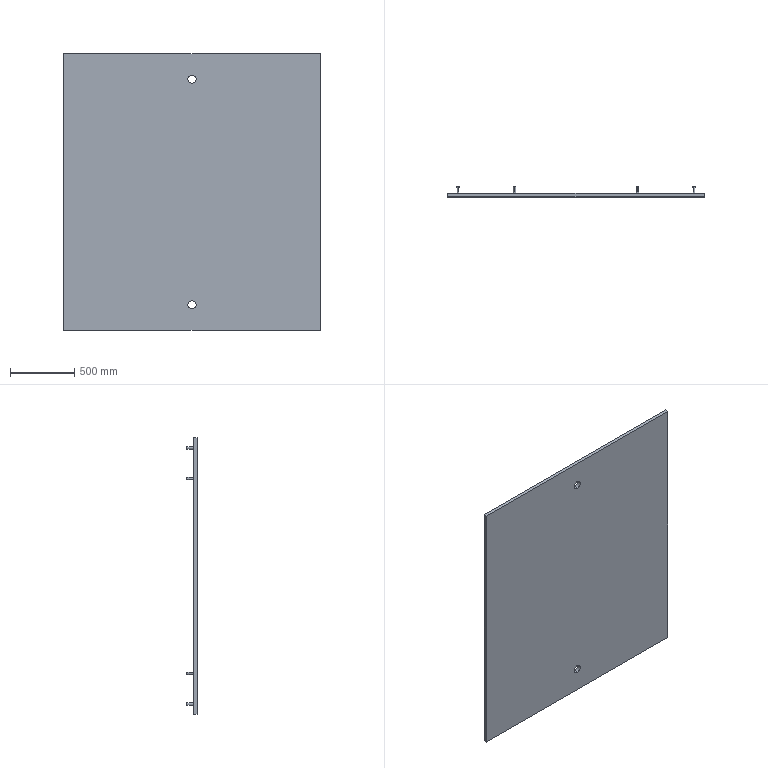Part | SolidWorks | features ICE 2, Extrusion 1 | 1 solid | 58 faces | box 2000 x 80 x 2160 mm | volume 129658308 mm3 | cylinder 36 | plane 22 | commonest cylinder face diameters 20 x32 64 x4
STEP:
#1=CARTESIAN_POINT('',(0.,0.,-848.));
#2=VERTEX_POINT('',#1);
#3=CARTESIAN_POINT('',(0.,0.,-912.));
#4=VERTEX_POINT('',#3);
#5=CARTESIAN_POINT('',(0.,0.,-880.));
#6=DIRECTION('',(0.,-1.,0.));
#7=DIRECTION('',(0.,0.,-1.));
#8=AXIS2_PLACEMENT_3D('',#5,#6,#7);
#9=CIRCLE('',#8,32.);
#10=EDGE_CURVE('',#2,#4,#9,.T.);
#11=ORIENTED_EDGE('',*,*,#10,.T.);
#12=CARTESIAN_POINT('',(0.,30.,-912.));
#13=VERTEX_POINT('',#12);
#14=CARTESIAN_POINT('',(0.,-10.,-912.));
#15=DIRECTION('',(0.,1.,0.));
#16=VECTOR('',#15,1000.);
#17=LINE('',#14,#16);
#18=EDGE_CURVE('',#4,#13,#17,.T.);
#19=ORIENTED_EDGE('',*,*,#18,.T.);
#20=CARTESIAN_POINT('',(0.,30.,-848.));
#21=VERTEX_POINT('',#20);
#22=CARTESIAN_POINT('',(0.,30.,-880.));
#23=DIRECTION('',(0.,1.,0.));
#24=DIRECTION('',(0.,0.,1.));
#25=AXIS2_PLACEMENT_3D('',#22,#23,#24);
#26=CIRCLE('',#25,32.);
#27=EDGE_CURVE('',#13,#21,#26,.T.);
#28=ORIENTED_EDGE('',*,*,#27,.T.);
#29=CARTESIAN_POINT('',(0.,-10.,-848.));
#30=DIRECTION('',(0.,1.,0.));
#31=VECTOR('',#30,1000.);
#32=LINE('',#29,#31);
#33=EDGE_CURVE('',#2,#21,#32,.T.);
#34=ORIENTED_EDGE('',*,*,#33,.F.);
#35=EDGE_LOOP('',(#11,#19,#28,#34));
#36=FACE_OUTER_BOUND('',#35,.T.);
#37=CARTESIAN_POINT('',(0.,-10.,-880.));
#38=DIRECTION('',(0.,1.,0.));
#39=DIRECTION('',(0.,0.,1.));
#40=AXIS2_PLACEMENT_3D('',#37,#38,#39);
#41=CYLINDRICAL_SURFACE('',#40,32.);
#42=ADVANCED_FACE('',(#36),#41,.F.);
#43=CARTESIAN_POINT('',(0.,0.,912.));
#44=VERTEX_POINT('',#43);
#45=CARTESIAN_POINT('',(0.,0.,848.));
#46=VERTEX_POINT('',#45);
#47=CARTESIAN_POINT('',(0.,0.,880.));
#48=DIRECTION('',(0.,-1.,0.));
#49=DIRECTION('',(0.,0.,-1.));
#50=AXIS2_PLACEMENT_3D('',#47,#48,#49);
#51=CIRCLE('',#50,32.);
#52=EDGE_CURVE('',#44,#46,#51,.T.);
#53=ORIENTED_EDGE('',*,*,#52,.T.);
#54=CARTESIAN_POINT('',(0.,30.,848.));
#55=VERTEX_POINT('',#54);
#56=CARTESIAN_POINT('',(0.,-10.,848.));
#57=DIRECTION('',(0.,1.,0.));
#58=VECTOR('',#57,1000.);
#59=LINE('',#56,#58);
#60=EDGE_CURVE('',#46,#55,#59,.T.);
#61=ORIENTED_EDGE('',*,*,#60,.T.);
#62=CARTESIAN_POINT('',(0.,30.,912.));
#63=VERTEX_POINT('',#62);
#64=CARTESIAN_POINT('',(0.,30.,880.));
#65=DIRECTION('',(0.,1.,0.));
#66=DIRECTION('',(0.,0.,1.));
#67=AXIS2_PLACEMENT_3D('',#64,#65,#66);
#68=CIRCLE('',#67,32.);
#69=EDGE_CURVE('',#55,#63,#68,.T.);
#70=ORIENTED_EDGE('',*,*,#69,.T.);
#71=CARTESIAN_POINT('',(0.,-10.,912.));
#72=DIRECTION('',(0.,1.,0.));
#73=VECTOR('',#72,1000.);
#74=LINE('',#71,#73);
#75=EDGE_CURVE('',#44,#63,#74,.T.);
#76=ORIENTED_EDGE('',*,*,#75,.F.);
#77=EDGE_LOOP('',(#53,#61,#70,#76));
#78=FACE_OUTER_BOUND('',#77,.T.);
#79=CARTESIAN_POINT('',(0.,-10.,880.));
#80=DIRECTION('',(0.,1.,0.));
#81=DIRECTION('',(0.,0.,1.));
#82=AXIS2_PLACEMENT_3D('',#79,#80,#81);
#83=CYLINDRICAL_SURFACE('',#82,32.);
#84=ADVANCED_FACE('',(#78),#83,.F.);
#85=CARTESIAN_POINT('',(-920.,80.,1010.));
#86=VERTEX_POINT('',#85);
#87=CARTESIAN_POINT('',(-920.,80.,990.));
#88=VERTEX_POINT('',#87);
#89=CARTESIAN_POINT('',(-920.,80.,1000.));
#90=DIRECTION('',(0.,1.,0.));
#91=DIRECTION('',(0.,0.,-1.));
#92=AXIS2_PLACEMENT_3D('',#89,#90,#91);
#93=CIRCLE('',#92,10.);
#94=EDGE_CURVE('',#86,#88,#93,.T.);
#95=ORIENTED_EDGE('',*,*,#94,.F.);
#96=CARTESIAN_POINT('',(-920.,30.,1010.));
#97=VERTEX_POINT('',#96);
#98=CARTESIAN_POINT('',(-920.,80.,1010.));
#99=DIRECTION('',(0.,-1.,0.));
#100=VECTOR('',#99,1000.);
#101=LINE('',#98,#100);
#102=EDGE_CURVE('',#86,#97,#101,.T.);
#103=ORIENTED_EDGE('',*,*,#102,.T.);
#104=CARTESIAN_POINT('',(-920.,30.,990.));
#105=VERTEX_POINT('',#104);
#106=CARTESIAN_POINT('',(-920.,30.,1000.));
#107=DIRECTION('',(0.,1.,0.));
#108=DIRECTION('',(0.,0.,-1.));
#109=AXIS2_PLACEMENT_3D('',#106,#107,#108);
#110=CIRCLE('',#109,10.);
#111=EDGE_CURVE('',#97,#105,#110,.T.);
#112=ORIENTED_EDGE('',*,*,#111,.T.);
#113=CARTESIAN_POINT('',(-920.,80.,990.));
#114=DIRECTION('',(0.,-1.,0.));
#115=VECTOR('',#114,1000.);
#116=LINE('',#113,#115);
#117=EDGE_CURVE('',#88,#105,#116,.T.);
#118=ORIENTED_EDGE('',*,*,#117,.F.);
#119=EDGE_LOOP('',(#95,#103,#112,#118));
#120=FACE_OUTER_BOUND('',#119,.T.);
#121=CARTESIAN_POINT('',(-920.,80.,1000.));
#122=DIRECTION('',(0.,-1.,0.));
#123=DIRECTION('',(0.,0.,-1.));
#124=AXIS2_PLACEMENT_3D('',#121,#122,#123);
#125=CYLINDRICAL_SURFACE('',#124,10.);
#126=ADVANCED_FACE('',(#120),#125,.T.);
#127=CARTESIAN_POINT('',(-920.,80.,770.));
#128=VERTEX_POINT('',#127);
#129=CARTESIAN_POINT('',(-920.,80.,750.));
#130=VERTEX_POINT('',#129);
#131=CARTESIAN_POINT('',(-920.,80.,760.));
#132=DIRECTION('',(0.,1.,0.));
#133=DIRECTION('',(0.,0.,-1.));
#134=AXIS2_PLACEMENT_3D('',#131,#132,#133);
#135=CIRCLE('',#134,10.);
#136=EDGE_CURVE('',#128,#130,#135,.T.);
#137=ORIENTED_EDGE('',*,*,#136,.F.);
#138=CARTESIAN_POINT('',(-920.,30.,770.));
#139=VERTEX_POINT('',#138);
#140=CARTESIAN_POINT('',(-920.,80.,770.));
#141=DIRECTION('',(0.,-1.,0.));
#142=VECTOR('',#141,1000.);
#143=LINE('',#140,#142);
#144=EDGE_CURVE('',#128,#139,#143,.T.);
#145=ORIENTED_EDGE('',*,*,#144,.T.);
#146=CARTESIAN_POINT('',(-920.,30.,750.));
#147=VERTEX_POINT('',#146);
#148=CARTESIAN_POINT('',(-920.,30.,760.));
#149=DIRECTION('',(0.,1.,0.));
#150=DIRECTION('',(0.,0.,-1.));
#151=AXIS2_PLACEMENT_3D('',#148,#149,#150);
#152=CIRCLE('',#151,10.);
#153=EDGE_CURVE('',#139,#147,#152,.T.);
#154=ORIENTED_EDGE('',*,*,#153,.T.);
#155=CARTESIAN_POINT('',(-920.,80.,750.));
#156=DIRECTION('',(0.,-1.,0.));
#157=VECTOR('',#156,1000.);
#158=LINE('',#155,#157);
#159=EDGE_CURVE('',#130,#147,#158,.T.);
#160=ORIENTED_EDGE('',*,*,#159,.F.);
#161=EDGE_LOOP('',(#137,#145,#154,#160));
#162=FACE_OUTER_BOUND('',#161,.T.);
#163=CARTESIAN_POINT('',(-920.,80.,760.));
#164=DIRECTION('',(0.,-1.,0.));
#165=DIRECTION('',(0.,0.,-1.));
#166=AXIS2_PLACEMENT_3D('',#163,#164,#165);
#167=CYLINDRICAL_SURFACE('',#166,10.);
#168=ADVANCED_FACE('',(#162),#167,.T.);
#169=CARTESIAN_POINT('',(-480.,80.,1010.));
#170=VERTEX_POINT('',#169);
#171=CARTESIAN_POINT('',(-480.,80.,990.));
#172=VERTEX_POINT('',#171);
#173=CARTESIAN_POINT('',(-480.,80.,1000.));
#174=DIRECTION('',(0.,1.,0.));
#175=DIRECTION('',(0.,0.,-1.));
#176=AXIS2_PLACEMENT_3D('',#173,#174,#175);
#177=CIRCLE('',#176,10.);
#178=EDGE_CURVE('',#170,#172,#177,.T.);
#179=ORIENTED_EDGE('',*,*,#178,.F.);
#180=CARTESIAN_POINT('',(-480.,30.,1010.));
#181=VERTEX_POINT('',#180);
#182=CARTESIAN_POINT('',(-480.,80.,1010.));
#183=DIRECTION('',(0.,-1.,0.));
#184=VECTOR('',#183,1000.);
#185=LINE('',#182,#184);
#186=EDGE_CURVE('',#170,#181,#185,.T.);
#187=ORIENTED_EDGE('',*,*,#186,.T.);
#188=CARTESIAN_POINT('',(-480.,30.,990.));
#189=VERTEX_POINT('',#188);
#190=CARTESIAN_POINT('',(-480.,30.,1000.));
#191=DIRECTION('',(0.,1.,0.));
#192=DIRECTION('',(0.,0.,-1.));
#193=AXIS2_PLACEMENT_3D('',#190,#191,#192);
#194=CIRCLE('',#193,10.);
#195=EDGE_CURVE('',#181,#189,#194,.T.);
#196=ORIENTED_EDGE('',*,*,#195,.T.);
#197=CARTESIAN_POINT('',(-480.,80.,990.));
#198=DIRECTION('',(0.,-1.,0.));
#199=VECTOR('',#198,1000.);
#200=LINE('',#197,#199);
#201=EDGE_CURVE('',#172,#189,#200,.T.);
#202=ORIENTED_EDGE('',*,*,#201,.F.);
#203=EDGE_LOOP('',(#179,#187,#196,#202));
#204=FACE_OUTER_BOUND('',#203,.T.);
#205=CARTESIAN_POINT('',(-480.,80.,1000.));
#206=DIRECTION('',(0.,-1.,0.));
#207=DIRECTION('',(0.,0.,-1.));
#208=AXIS2_PLACEMENT_3D('',#205,#206,#207);
#209=CYLINDRICAL_SURFACE('',#208,10.);
#210=ADVANCED_FACE('',(#204),#209,.T.);
#211=CARTESIAN_POINT('',(-480.,80.,770.));
#212=VERTEX_POINT('',#211);
#213=CARTESIAN_POINT('',(-480.,80.,750.));
#214=VERTEX_POINT('',#213);
#215=CARTESIAN_POINT('',(-480.,80.,760.));
#216=DIRECTION('',(0.,1.,0.));
#217=DIRECTION('',(0.,0.,-1.));
#218=AXIS2_PLACEMENT_3D('',#215,#216,#217);
#219=CIRCLE('',#218,10.);
#220=EDGE_CURVE('',#212,#214,#219,.T.);
#221=ORIENTED_EDGE('',*,*,#220,.F.);
#222=CARTESIAN_POINT('',(-480.,30.,770.));
#223=VERTEX_POINT('',#222);
#224=CARTESIAN_POINT('',(-480.,80.,770.));
#225=DIRECTION('',(0.,-1.,0.));
#226=VECTOR('',#225,1000.);
#227=LINE('',#224,#226);
#228=EDGE_CURVE('',#212,#223,#227,.T.);
#229=ORIENTED_EDGE('',*,*,#228,.T.);
#230=CARTESIAN_POINT('',(-480.,30.,750.));
#231=VERTEX_POINT('',#230);
#232=CARTESIAN_POINT('',(-480.,30.,760.));
#233=DIRECTION('',(0.,1.,0.));
#234=DIRECTION('',(0.,0.,-1.));
#235=AXIS2_PLACEMENT_3D('',#232,#233,#234);
#236=CIRCLE('',#235,10.);
#237=EDGE_CURVE('',#223,#231,#236,.T.);
#238=ORIENTED_EDGE('',*,*,#237,.T.);
#239=CARTESIAN_POINT('',(-480.,80.,750.));
#240=DIRECTION('',(0.,-1.,0.));
#241=VECTOR('',#240,1000.);
#242=LINE('',#239,#241);
#243=EDGE_CURVE('',#214,#231,#242,.T.);
#244=ORIENTED_EDGE('',*,*,#243,.F.);
#245=EDGE_LOOP('',(#221,#229,#238,#244));
#246=FACE_OUTER_BOUND('',#245,.T.);
#247=CARTESIAN_POINT('',(-480.,80.,760.));
#248=DIRECTION('',(0.,-1.,0.));
#249=DIRECTION('',(0.,0.,-1.));
#250=AXIS2_PLACEMENT_3D('',#247,#248,#249);
#251=CYLINDRICAL_SURFACE('',#250,10.);
#252=ADVANCED_FACE('',(#246),#251,.T.);
#253=CARTESIAN_POINT('',(480.,80.,770.));
#254=VERTEX_POINT('',#253);
#255=CARTESIAN_POINT('',(480.,80.,750.));
#256=VERTEX_POINT('',#255);
#257=CARTESIAN_POINT('',(480.,80.,760.));
#258=DIRECTION('',(0.,1.,0.));
#259=DIRECTION('',(0.,0.,1.));
#260=AXIS2_PLACEMENT_3D('',#257,#258,#259);
#261=CIRCLE('',#260,10.);
#262=EDGE_CURVE('',#254,#256,#261,.T.);
#263=ORIENTED_EDGE('',*,*,#262,.F.);
#264=CARTESIAN_POINT('',(480.,30.,770.));
#265=VERTEX_POINT('',#264);
#266=CARTESIAN_POINT('',(480.,80.,770.));
#267=DIRECTION('',(0.,-1.,0.));
#268=VECTOR('',#267,1000.);
#269=LINE('',#266,#268);
#270=EDGE_CURVE('',#254,#265,#269,.T.);
#271=ORIENTED_EDGE('',*,*,#270,.T.);
#272=CARTESIAN_POINT('',(480.,30.,750.));
#273=VERTEX_POINT('',#272);
#274=CARTESIAN_POINT('',(480.,30.,760.));
#275=DIRECTION('',(0.,1.,0.));
#276=DIRECTION('',(0.,0.,-1.));
#277=AXIS2_PLACEMENT_3D('',#274,#275,#276);
#278=CIRCLE('',#277,10.);
#279=EDGE_CURVE('',#265,#273,#278,.T.);
#280=ORIENTED_EDGE('',*,*,#279,.T.);
#281=CARTESIAN_POINT('',(480.,80.,750.));
#282=DIRECTION('',(0.,-1.,0.));
#283=VECTOR('',#282,1000.);
#284=LINE('',#281,#283);
#285=EDGE_CURVE('',#256,#273,#284,.T.);
#286=ORIENTED_EDGE('',*,*,#285,.F.);
#287=EDGE_LOOP('',(#263,#271,#280,#286));
#288=FACE_OUTER_BOUND('',#287,.T.);
#289=CARTESIAN_POINT('',(480.,80.,760.));
#290=DIRECTION('',(0.,-1.,0.));
#291=DIRECTION('',(0.,0.,-1.));
#292=AXIS2_PLACEMENT_3D('',#289,#290,#291);
#293=CYLINDRICAL_SURFACE('',#292,10.);
#294=ADVANCED_FACE('',(#288),#293,.T.);
#295=CARTESIAN_POINT('',(480.,80.,1010.));
#296=VERTEX_POINT('',#295);
#297=CARTESIAN_POINT('',(480.,80.,990.));
#298=VERTEX_POINT('',#297);
#299=CARTESIAN_POINT('',(480.,80.,1000.));
#300=DIRECTION('',(0.,1.,0.));
#301=DIRECTION('',(0.,0.,1.));
#302=AXIS2_PLACEMENT_3D('',#299,#300,#301);
#303=CIRCLE('',#302,10.);
#304=EDGE_CURVE('',#296,#298,#303,.T.);
#305=ORIENTED_EDGE('',*,*,#304,.F.);
#306=CARTESIAN_POINT('',(480.,30.,1010.));
#307=VERTEX_POINT('',#306);
#308=CARTESIAN_POINT('',(480.,80.,1010.));
#309=DIRECTION('',(0.,-1.,0.));
#310=VECTOR('',#309,1000.);
#311=LINE('',#308,#310);
#312=EDGE_CURVE('',#296,#307,#311,.T.);
#313=ORIENTED_EDGE('',*,*,#312,.T.);
#314=CARTESIAN_POINT('',(480.,30.,990.));
#315=VERTEX_POINT('',#314);
#316=CARTESIAN_POINT('',(480.,30.,1000.));
#317=DIRECTION('',(0.,1.,0.));
#318=DIRECTION('',(0.,0.,-1.));
#319=AXIS2_PLACEMENT_3D('',#316,#317,#318);
#320=CIRCLE('',#319,10.);
#321=EDGE_CURVE('',#307,#315,#320,.T.);
#322=ORIENTED_EDGE('',*,*,#321,.T.);
#323=CARTESIAN_POINT('',(480.,80.,990.));
#324=DIRECTION('',(0.,-1.,0.));
#325=VECTOR('',#324,1000.);
#326=LINE('',#323,#325);
#327=EDGE_CURVE('',#298,#315,#326,.T.);
#328=ORIENTED_EDGE('',*,*,#327,.F.);
#329=EDGE_LOOP('',(#305,#313,#322,#328));
#330=FACE_OUTER_BOUND('',#329,.T.);
#331=CARTESIAN_POINT('',(480.,80.,1000.));
#332=DIRECTION('',(0.,-1.,0.));
#333=DIRECTION('',(0.,0.,-1.));
#334=AXIS2_PLACEMENT_3D('',#331,#332,#333);
#335=CYLINDRICAL_SURFACE('',#334,10.);
#336=ADVANCED_FACE('',(#330),#335,.T.);
#337=CARTESIAN_POINT('',(920.,80.,770.));
#338=VERTEX_POINT('',#337);
#339=CARTESIAN_POINT('',(920.,80.,750.));
#340=VERTEX_POINT('',#339);
#341=CARTESIAN_POINT('',(920.,80.,760.));
#342=DIRECTION('',(0.,1.,0.));
#343=DIRECTION('',(0.,0.,1.));
#344=AXIS2_PLACEMENT_3D('',#341,#342,#343);
#345=CIRCLE('',#344,10.);
#346=EDGE_CURVE('',#338,#340,#345,.T.);
#347=ORIENTED_EDGE('',*,*,#346,.F.);
#348=CARTESIAN_POINT('',(920.,30.,770.));
#349=VERTEX_POINT('',#348);
#350=CARTESIAN_POINT('',(920.,80.,770.));
#351=DIRECTION('',(0.,-1.,0.));
#352=VECTOR('',#351,1000.);
#353=LINE('',#350,#352);
#354=EDGE_CURVE('',#338,#349,#353,.T.);
#355=ORIENTED_EDGE('',*,*,#354,.T.);
#356=CARTESIAN_POINT('',(920.,30.,750.));
#357=VERTEX_POINT('',#356);
#358=CARTESIAN_POINT('',(920.,30.,760.));
#359=DIRECTION('',(0.,1.,0.));
#360=DIRECTION('',(0.,0.,-1.));
#361=AXIS2_PLACEMENT_3D('',#358,#359,#360);
#362=CIRCLE('',#361,10.);
#363=EDGE_CURVE('',#349,#357,#362,.T.);
#364=ORIENTED_EDGE('',*,*,#363,.T.);
#365=CARTESIAN_POINT('',(920.,80.,750.));
#366=DIRECTION('',(0.,-1.,0.));
#367=VECTOR('',#366,1000.);
#368=LINE('',#365,#367);
#369=EDGE_CURVE('',#340,#357,#368,.T.);
#370=ORIENTED_EDGE('',*,*,#369,.F.);
#371=EDGE_LOOP('',(#347,#355,#364,#370));
#372=FACE_OUTER_BOUND('',#371,.T.);
#373=CARTESIAN_POINT('',(920.,80.,760.));
#374=DIRECTION('',(0.,-1.,0.));
#375=DIRECTION('',(0.,0.,-1.));
#376=AXIS2_PLACEMENT_3D('',#373,#374,#375);
#377=CYLINDRICAL_SURFACE('',#376,10.);
#378=ADVANCED_FACE('',(#372),#377,.T.);
#379=CARTESIAN_POINT('',(920.,80.,1010.));
#380=VERTEX_POINT('',#379);
#381=CARTESIAN_POINT('',(920.,80.,990.));
#382=VERTEX_POINT('',#381);
#383=CARTESIAN_POINT('',(920.,80.,1000.));
#384=DIRECTION('',(0.,1.,0.));
#385=DIRECTION('',(0.,0.,1.));
#386=AXIS2_PLACEMENT_3D('',#383,#384,#385);
#387=CIRCLE('',#386,10.);
#388=EDGE_CURVE('',#380,#382,#387,.T.);
#389=ORIENTED_EDGE('',*,*,#388,.F.);
#390=CARTESIAN_POINT('',(920.,30.,1010.));
#391=VERTEX_POINT('',#390);
#392=CARTESIAN_POINT('',(920.,80.,1010.));
#393=DIRECTION('',(0.,-1.,0.));
#394=VECTOR('',#393,1000.);
#395=LINE('',#392,#394);
#396=EDGE_CURVE('',#380,#391,#395,.T.);
#397=ORIENTED_EDGE('',*,*,#396,.T.);
#398=CARTESIAN_POINT('',(920.,30.,990.));
#399=VERTEX_POINT('',#398);
#400=CARTESIAN_POINT('',(920.,30.,1000.));
#401=DIRECTION('',(0.,1.,0.));
#402=DIRECTION('',(0.,0.,-1.));
#403=AXIS2_PLACEMENT_3D('',#400,#401,#402);
#404=CIRCLE('',#403,10.);
#405=EDGE_CURVE('',#391,#399,#404,.T.);
#406=ORIENTED_EDGE('',*,*,#405,.T.);
#407=CARTESIAN_POINT('',(920.,80.,990.));
#408=DIRECTION('',(0.,-1.,0.));
#409=VECTOR('',#408,1000.);
#410=LINE('',#407,#409);
#411=EDGE_CURVE('',#382,#399,#410,.T.);
#412=ORIENTED_EDGE('',*,*,#411,.F.);
#413=EDGE_LOOP('',(#389,#397,#406,#412));
#414=FACE_OUTER_BOUND('',#413,.T.);
#415=CARTESIAN_POINT('',(920.,80.,1000.));
#416=DIRECTION('',(0.,-1.,0.));
#417=DIRECTION('',(0.,0.,-1.));
#418=AXIS2_PLACEMENT_3D('',#415,#416,#417);
#419=CYLINDRICAL_SURFACE('',#418,10.);
#420=ADVANCED_FACE('',(#414),#419,.T.);
#421=CARTESIAN_POINT('',(920.,80.,-990.));
#422=VERTEX_POINT('',#421);
#423=CARTESIAN_POINT('',(920.,80.,-1010.));
#424=VERTEX_POINT('',#423);
#425=CARTESIAN_POINT('',(920.,80.,-1000.));
#426=DIRECTION('',(0.,1.,0.));
#427=DIRECTION('',(0.,0.,-1.));
#428=AXIS2_PLACEMENT_3D('',#425,#426,#427);
#429=CIRCLE('',#428,10.);
#430=EDGE_CURVE('',#422,#424,#429,.T.);
#431=ORIENTED_EDGE('',*,*,#430,.F.);
#432=CARTESIAN_POINT('',(920.,30.,-990.));
#433=VERTEX_POINT('',#432);
#434=CARTESIAN_POINT('',(920.,80.,-990.));
#435=DIRECTION('',(0.,-1.,0.));
#436=VECTOR('',#435,1000.);
#437=LINE('',#434,#436);
#438=EDGE_CURVE('',#422,#433,#437,.T.);
#439=ORIENTED_EDGE('',*,*,#438,.T.);
#440=CARTESIAN_POINT('',(920.,30.,-1010.));
#441=VERTEX_POINT('',#440);
#442=CARTESIAN_POINT('',(920.,30.,-1000.));
#443=DIRECTION('',(0.,1.,0.));
#444=DIRECTION('',(0.,0.,-1.));
#445=AXIS2_PLACEMENT_3D('',#442,#443,#444);
#446=CIRCLE('',#445,10.);
#447=EDGE_CURVE('',#433,#441,#446,.T.);
#448=ORIENTED_EDGE('',*,*,#447,.T.);
#449=CARTESIAN_POINT('',(920.,80.,-1010.));
#450=DIRECTION('',(0.,-1.,0.));
#451=VECTOR('',#450,1000.);
#452=LINE('',#449,#451);
#453=EDGE_CURVE('',#424,#441,#452,.T.);
#454=ORIENTED_EDGE('',*,*,#453,.F.);
#455=EDGE_LOOP('',(#431,#439,#448,#454));
#456=FACE_OUTER_BOUND('',#455,.T.);
#457=CARTESIAN_POINT('',(920.,80.,-1000.));
#458=DIRECTION('',(0.,-1.,0.));
#459=DIRECTION('',(0.,0.,-1.));
#460=AXIS2_PLACEMENT_3D('',#457,#458,#459);
#461=CYLINDRICAL_SURFACE('',#460,10.);
#462=ADVANCED_FACE('',(#456),#461,.T.);
#463=CARTESIAN_POINT('',(920.,80.,-750.));
#464=VERTEX_POINT('',#463);
#465=CARTESIAN_POINT('',(920.,80.,-770.));
#466=VERTEX_POINT('',#465);
#467=CARTESIAN_POINT('',(920.,80.,-760.));
#468=DIRECTION('',(0.,1.,0.));
#469=DIRECTION('',(0.,0.,-1.));
#470=AXIS2_PLACEMENT_3D('',#467,#468,#469);
#471=CIRCLE('',#470,10.);
#472=EDGE_CURVE('',#464,#466,#471,.T.);
#473=ORIENTED_EDGE('',*,*,#472,.F.);
#474=CARTESIAN_POINT('',(920.,30.,-750.));
#475=VERTEX_POINT('',#474);
#476=CARTESIAN_POINT('',(920.,80.,-750.));
#477=DIRECTION('',(0.,-1.,0.));
#478=VECTOR('',#477,1000.);
#479=LINE('',#476,#478);
#480=EDGE_CURVE('',#464,#475,#479,.T.);
#481=ORIENTED_EDGE('',*,*,#480,.T.);
#482=CARTESIAN_POINT('',(920.,30.,-770.));
#483=VERTEX_POINT('',#482);
#484=CARTESIAN_POINT('',(920.,30.,-760.));
#485=DIRECTION('',(0.,1.,0.));
#486=DIRECTION('',(0.,0.,-1.));
#487=AXIS2_PLACEMENT_3D('',#484,#485,#486);
#488=CIRCLE('',#487,10.);
#489=EDGE_CURVE('',#475,#483,#488,.T.);
#490=ORIENTED_EDGE('',*,*,#489,.T.);
#491=CARTESIAN_POINT('',(920.,80.,-770.));
#492=DIRECTION('',(0.,-1.,0.));
#493=VECTOR('',#492,1000.);
#494=LINE('',#491,#493);
#495=EDGE_CURVE('',#466,#483,#494,.T.);
#496=ORIENTED_EDGE('',*,*,#495,.F.);
#497=EDGE_LOOP('',(#473,#481,#490,#496));
#498=FACE_OUTER_BOUND('',#497,.T.);
#499=CARTESIAN_POINT('',(920.,80.,-760.));
#500=DIRECTION('',(0.,-1.,0.));
#501=DIRECTION('',(0.,0.,-1.));
#502=AXIS2_PLACEMENT_3D('',#499,#500,#501);
#503=CYLINDRICAL_SURFACE('',#502,10.);
#504=ADVANCED_FACE('',(#498),#503,.T.);
#505=CARTESIAN_POINT('',(480.,80.,-990.));
#506=VERTEX_POINT('',#505);
#507=CARTESIAN_POINT('',(480.,80.,-1010.));
#508=VERTEX_POINT('',#507);
#509=CARTESIAN_POINT('',(480.,80.,-1000.));
#510=DIRECTION('',(0.,1.,0.));
#511=DIRECTION('',(0.,0.,-1.));
#512=AXIS2_PLACEMENT_3D('',#509,#510,#511);
#513=CIRCLE('',#512,10.);
#514=EDGE_CURVE('',#506,#508,#513,.T.);
#515=ORIENTED_EDGE('',*,*,#514,.F.);
#516=CARTESIAN_POINT('',(480.,30.,-990.));
#517=VERTEX_POINT('',#516);
#518=CARTESIAN_POINT('',(480.,80.,-990.));
#519=DIRECTION('',(0.,-1.,0.));
#520=VECTOR('',#519,1000.);
#521=LINE('',#518,#520);
#522=EDGE_CURVE('',#506,#517,#521,.T.);
#523=ORIENTED_EDGE('',*,*,#522,.T.);
#524=CARTESIAN_POINT('',(480.,30.,-1010.));
#525=VERTEX_POINT('',#524);
#526=CARTESIAN_POINT('',(480.,30.,-1000.));
#527=DIRECTION('',(0.,1.,0.));
#528=DIRECTION('',(0.,0.,-1.));
#529=AXIS2_PLACEMENT_3D('',#526,#527,#528);
#530=CIRCLE('',#529,10.);
#531=EDGE_CURVE('',#517,#525,#530,.T.);
#532=ORIENTED_EDGE('',*,*,#531,.T.);
#533=CARTESIAN_POINT('',(480.,80.,-1010.));
#534=DIRECTION('',(0.,-1.,0.));
#535=VECTOR('',#534,1000.);
#536=LINE('',#533,#535);
#537=EDGE_CURVE('',#508,#525,#536,.T.);
#538=ORIENTED_EDGE('',*,*,#537,.F.);
#539=EDGE_LOOP('',(#515,#523,#532,#538));
#540=FACE_OUTER_BOUND('',#539,.T.);
#541=CARTESIAN_POINT('',(480.,80.,-1000.));
#542=DIRECTION('',(0.,-1.,0.));
#543=DIRECTION('',(0.,0.,-1.));
#544=AXIS2_PLACEMENT_3D('',#541,#542,#543);
#545=CYLINDRICAL_SURFACE('',#544,10.);
#546=ADVANCED_FACE('',(#540),#545,.T.);
#547=CARTESIAN_POINT('',(480.,80.,-750.));
#548=VERTEX_POINT('',#547);
#549=CARTESIAN_POINT('',(480.,80.,-770.));
#550=VERTEX_POINT('',#549);
#551=CARTESIAN_POINT('',(480.,80.,-760.));
#552=DIRECTION('',(0.,1.,0.));
#553=DIRECTION('',(0.,0.,-1.));
#554=AXIS2_PLACEMENT_3D('',#551,#552,#553);
#555=CIRCLE('',#554,10.);
#556=EDGE_CURVE('',#548,#550,#555,.T.);
#557=ORIENTED_EDGE('',*,*,#556,.F.);
#558=CARTESIAN_POINT('',(480.,30.,-750.));
#559=VERTEX_POINT('',#558);
#560=CARTESIAN_POINT('',(480.,80.,-750.));
#561=DIRECTION('',(0.,-1.,0.));
#562=VECTOR('',#561,1000.);
#563=LINE('',#560,#562);
#564=EDGE_CURVE('',#548,#559,#563,.T.);
#565=ORIENTED_EDGE('',*,*,#564,.T.);
#566=CARTESIAN_POINT('',(480.,30.,-770.));
#567=VERTEX_POINT('',#566);
#568=CARTESIAN_POINT('',(480.,30.,-760.));
#569=DIRECTION('',(0.,1.,0.));
#570=DIRECTION('',(0.,0.,-1.));
#571=AXIS2_PLACEMENT_3D('',#568,#569,#570);
#572=CIRCLE('',#571,10.);
#573=EDGE_CURVE('',#559,#567,#572,.T.);
#574=ORIENTED_EDGE('',*,*,#573,.T.);
#575=CARTESIAN_POINT('',(480.,80.,-770.));
#576=DIRECTION('',(0.,-1.,0.));
#577=VECTOR('',#576,1000.);
#578=LINE('',#575,#577);
#579=EDGE_CURVE('',#550,#567,#578,.T.);
#580=ORIENTED_EDGE('',*,*,#579,.F.);
#581=EDGE_LOOP('',(#557,#565,#574,#580));
#582=FACE_OUTER_BOUND('',#581,.T.);
#583=CARTESIAN_POINT('',(480.,80.,-760.));
#584=DIRECTION('',(0.,-1.,0.));
#585=DIRECTION('',(0.,0.,-1.));
#586=AXIS2_PLACEMENT_3D('',#583,#584,#585);
#587=CYLINDRICAL_SURFACE('',#586,10.);
#588=ADVANCED_FACE('',(#582),#587,.T.);
#589=CARTESIAN_POINT('',(-480.,80.,-750.));
#590=VERTEX_POINT('',#589);
#591=CARTESIAN_POINT('',(-480.,80.,-770.));
#592=VERTEX_POINT('',#591);
#593=CARTESIAN_POINT('',(-480.,80.,-760.));
#594=DIRECTION('',(0.,1.,0.));
#595=DIRECTION('',(0.,0.,1.));
#596=AXIS2_PLACEMENT_3D('',#593,#594,#595);
#597=CIRCLE('',#596,10.);
#598=EDGE_CURVE('',#590,#592,#597,.T.);
#599=ORIENTED_EDGE('',*,*,#598,.F.);
#600=CARTESIAN_POINT('',(-480.,30.,-750.));
#601=VERTEX_POINT('',#600);
#602=CARTESIAN_POINT('',(-480.,80.,-750.));
#603=DIRECTION('',(0.,-1.,0.));
#604=VECTOR('',#603,1000.);
#605=LINE('',#602,#604);
#606=EDGE_CURVE('',#590,#601,#605,.T.);
#607=ORIENTED_EDGE('',*,*,#606,.T.);
#608=CARTESIAN_POINT('',(-480.,30.,-770.));
#609=VERTEX_POINT('',#608);
#610=CARTESIAN_POINT('',(-480.,30.,-760.));
#611=DIRECTION('',(0.,1.,0.));
#612=DIRECTION('',(0.,0.,-1.));
#613=AXIS2_PLACEMENT_3D('',#610,#611,#612);
#614=CIRCLE('',#613,10.);
#615=EDGE_CURVE('',#601,#609,#614,.T.);
#616=ORIENTED_EDGE('',*,*,#615,.T.);
#617=CARTESIAN_POINT('',(-480.,80.,-770.));
#618=DIRECTION('',(0.,-1.,0.));
#619=VECTOR('',#618,1000.);
#620=LINE('',#617,#619);
#621=EDGE_CURVE('',#592,#609,#620,.T.);
#622=ORIENTED_EDGE('',*,*,#621,.F.);
#623=EDGE_LOOP('',(#599,#607,#616,#622));
#624=FACE_OUTER_BOUND('',#623,.T.);
#625=CARTESIAN_POINT('',(-480.,80.,-760.));
#626=DIRECTION('',(0.,-1.,0.));
#627=DIRECTION('',(0.,0.,-1.));
#628=AXIS2_PLACEMENT_3D('',#625,#626,#627);
#629=CYLINDRICAL_SURFACE('',#628,10.);
#630=ADVANCED_FACE('',(#624),#629,.T.);
#631=CARTESIAN_POINT('',(-480.,80.,-990.));
#632=VERTEX_POINT('',#631);
#633=CARTESIAN_POINT('',(-480.,80.,-1010.));
#634=VERTEX_POINT('',#633);
#635=CARTESIAN_POINT('',(-480.,80.,-1000.));
#636=DIRECTION('',(0.,1.,0.));
#637=DIRECTION('',(0.,0.,1.));
#638=AXIS2_PLACEMENT_3D('',#635,#636,#637);
#639=CIRCLE('',#638,10.);
#640=EDGE_CURVE('',#632,#634,#639,.T.);
#641=ORIENTED_EDGE('',*,*,#640,.F.);
#642=CARTESIAN_POINT('',(-480.,30.,-990.));
#643=VERTEX_POINT('',#642);
#644=CARTESIAN_POINT('',(-480.,80.,-990.));
#645=DIRECTION('',(0.,-1.,0.));
#646=VECTOR('',#645,1000.);
#647=LINE('',#644,#646);
#648=EDGE_CURVE('',#632,#643,#647,.T.);
#649=ORIENTED_EDGE('',*,*,#648,.T.);
#650=CARTESIAN_POINT('',(-480.,30.,-1010.));
#651=VERTEX_POINT('',#650);
#652=CARTESIAN_POINT('',(-480.,30.,-1000.));
#653=DIRECTION('',(0.,1.,0.));
#654=DIRECTION('',(0.,0.,-1.));
#655=AXIS2_PLACEMENT_3D('',#652,#653,#654);
#656=CIRCLE('',#655,10.);
#657=EDGE_CURVE('',#643,#651,#656,.T.);
#658=ORIENTED_EDGE('',*,*,#657,.T.);
#659=CARTESIAN_POINT('',(-480.,80.,-1010.));
#660=DIRECTION('',(0.,-1.,0.));
#661=VECTOR('',#660,1000.);
#662=LINE('',#659,#661);
#663=EDGE_CURVE('',#634,#651,#662,.T.);
#664=ORIENTED_EDGE('',*,*,#663,.F.);
#665=EDGE_LOOP('',(#641,#649,#658,#664));
#666=FACE_OUTER_BOUND('',#665,.T.);
#667=CARTESIAN_POINT('',(-480.,80.,-1000.));
#668=DIRECTION('',(0.,-1.,0.));
#669=DIRECTION('',(0.,0.,-1.));
#670=AXIS2_PLACEMENT_3D('',#667,#668,#669);
#671=CYLINDRICAL_SURFACE('',#670,10.);
#672=ADVANCED_FACE('',(#666),#671,.T.);
#673=CARTESIAN_POINT('',(-920.,80.,-750.));
#674=VERTEX_POINT('',#673);
#675=CARTESIAN_POINT('',(-920.,80.,-770.));
#676=VERTEX_POINT('',#675);
#677=CARTESIAN_POINT('',(-920.,80.,-760.));
#678=DIRECTION('',(0.,1.,0.));
#679=DIRECTION('',(0.,0.,1.));
#680=AXIS2_PLACEMENT_3D('',#677,#678,#679);
#681=CIRCLE('',#680,10.);
#682=EDGE_CURVE('',#674,#676,#681,.T.);
#683=ORIENTED_EDGE('',*,*,#682,.F.);
#684=CARTESIAN_POINT('',(-920.,30.,-750.));
#685=VERTEX_POINT('',#684);
#686=CARTESIAN_POINT('',(-920.,80.,-750.));
#687=DIRECTION('',(0.,-1.,0.));
#688=VECTOR('',#687,1000.);
#689=LINE('',#686,#688);
#690=EDGE_CURVE('',#674,#685,#689,.T.);
#691=ORIENTED_EDGE('',*,*,#690,.T.);
#692=CARTESIAN_POINT('',(-920.,30.,-770.));
#693=VERTEX_POINT('',#692);
#694=CARTESIAN_POINT('',(-920.,30.,-760.));
#695=DIRECTION('',(0.,1.,0.));
#696=DIRECTION('',(0.,0.,-1.));
#697=AXIS2_PLACEMENT_3D('',#694,#695,#696);
#698=CIRCLE('',#697,10.);
#699=EDGE_CURVE('',#685,#693,#698,.T.);
#700=ORIENTED_EDGE('',*,*,#699,.T.);
#701=CARTESIAN_POINT('',(-920.,80.,-770.));
#702=DIRECTION('',(0.,-1.,0.));
#703=VECTOR('',#702,1000.);
#704=LINE('',#701,#703);
#705=EDGE_CURVE('',#676,#693,#704,.T.);
#706=ORIENTED_EDGE('',*,*,#705,.F.);
#707=EDGE_LOOP('',(#683,#691,#700,#706));
#708=FACE_OUTER_BOUND('',#707,.T.);
#709=CARTESIAN_POINT('',(-920.,80.,-760.));
#710=DIRECTION('',(0.,-1.,0.));
#711=DIRECTION('',(0.,0.,-1.));
#712=AXIS2_PLACEMENT_3D('',#709,#710,#711);
#713=CYLINDRICAL_SURFACE('',#712,10.);
#714=ADVANCED_FACE('',(#708),#713,.T.);
#715=CARTESIAN_POINT('',(-920.,80.,-990.));
#716=VERTEX_POINT('',#715);
#717=CARTESIAN_POINT('',(-920.,80.,-1010.));
#718=VERTEX_POINT('',#717);
#719=CARTESIAN_POINT('',(-920.,80.,-1000.));
#720=DIRECTION('',(0.,1.,0.));
#721=DIRECTION('',(0.,0.,1.));
#722=AXIS2_PLACEMENT_3D('',#719,#720,#721);
#723=CIRCLE('',#722,10.);
#724=EDGE_CURVE('',#716,#718,#723,.T.);
#725=ORIENTED_EDGE('',*,*,#724,.F.);
#726=CARTESIAN_POINT('',(-920.,30.,-990.));
#727=VERTEX_POINT('',#726);
#728=CARTESIAN_POINT('',(-920.,80.,-990.));
#729=DIRECTION('',(0.,-1.,0.));
#730=VECTOR('',#729,1000.);
#731=LINE('',#728,#730);
#732=EDGE_CURVE('',#716,#727,#731,.T.);
#733=ORIENTED_EDGE('',*,*,#732,.T.);
#734=CARTESIAN_POINT('',(-920.,30.,-1010.));
#735=VERTEX_POINT('',#734);
#736=CARTESIAN_POINT('',(-920.,30.,-1000.));
#737=DIRECTION('',(0.,1.,0.));
#738=DIRECTION('',(0.,0.,-1.));
#739=AXIS2_PLACEMENT_3D('',#736,#737,#738);
#740=CIRCLE('',#739,10.);
#741=EDGE_CURVE('',#727,#735,#740,.T.);
#742=ORIENTED_EDGE('',*,*,#741,.T.);
#743=CARTESIAN_POINT('',(-920.,80.,-1010.));
#744=DIRECTION('',(0.,-1.,0.));
#745=VECTOR('',#744,1000.);
#746=LINE('',#743,#745);
#747=EDGE_CURVE('',#718,#735,#746,.T.);
#748=ORIENTED_EDGE('',*,*,#747,.F.);
#749=EDGE_LOOP('',(#725,#733,#742,#748));
#750=FACE_OUTER_BOUND('',#749,.T.);
#751=CARTESIAN_POINT('',(-920.,80.,-1000.));
#752=DIRECTION('',(0.,-1.,0.));
#753=DIRECTION('',(0.,0.,-1.));
#754=AXIS2_PLACEMENT_3D('',#751,#752,#753);
#755=CYLINDRICAL_SURFACE('',#754,10.);
#756=ADVANCED_FACE('',(#750),#755,.T.);
#757=CARTESIAN_POINT('',(1000.,0.,1080.));
#758=VERTEX_POINT('',#757);
#759=CARTESIAN_POINT('',(1000.,0.,-1080.));
#760=VERTEX_POINT('',#759);
#761=CARTESIAN_POINT('',(1000.,0.,1080.));
#762=DIRECTION('',(0.,0.,-1.));
#763=VECTOR('',#762,1000.);
#764=LINE('',#761,#763);
#765=EDGE_CURVE('',#758,#760,#764,.T.);
#766=ORIENTED_EDGE('',*,*,#765,.T.);
#767=CARTESIAN_POINT('',(1000.,30.,-1080.));
#768=VERTEX_POINT('',#767);
#769=CARTESIAN_POINT('',(1000.,30.,-1080.));
#770=DIRECTION('',(0.,-1.,0.));
#771=VECTOR('',#770,1000.);
#772=LINE('',#769,#771);
#773=EDGE_CURVE('',#768,#760,#772,.T.);
#774=ORIENTED_EDGE('',*,*,#773,.F.);
#775=CARTESIAN_POINT('',(1000.,30.,1080.));
#776=VERTEX_POINT('',#775);
#777=CARTESIAN_POINT('',(1000.,30.,1080.));
#778=DIRECTION('',(0.,0.,-1.));
#779=VECTOR('',#778,1000.);
#780=LINE('',#777,#779);
#781=EDGE_CURVE('',#776,#768,#780,.T.);
#782=ORIENTED_EDGE('',*,*,#781,.F.);
#783=CARTESIAN_POINT('',(1000.,30.,1080.));
#784=DIRECTION('',(0.,-1.,0.));
#785=VECTOR('',#784,1000.);
#786=LINE('',#783,#785);
#787=EDGE_CURVE('',#776,#758,#786,.T.);
#788=ORIENTED_EDGE('',*,*,#787,.T.);
#789=EDGE_LOOP('',(#766,#774,#782,#788));
#790=FACE_OUTER_BOUND('',#789,.T.);
#791=CARTESIAN_POINT('',(1000.,30.,1080.));
#792=DIRECTION('',(-1.,0.,0.));
#793=DIRECTION('',(0.,0.,1.));
#794=AXIS2_PLACEMENT_3D('',#791,#792,#793);
#795=PLANE('',#794);
#796=ADVANCED_FACE('',(#790),#795,.F.);
#797=CARTESIAN_POINT('',(-1000.,0.,-1080.));
#798=VERTEX_POINT('',#797);
#799=CARTESIAN_POINT('',(-1000.,0.,-1080.));
#800=DIRECTION('',(-1.,0.,0.));
#801=VECTOR('',#800,1000.);
#802=LINE('',#799,#801);
#803=EDGE_CURVE('',#760,#798,#802,.T.);
#804=ORIENTED_EDGE('',*,*,#803,.T.);
#805=CARTESIAN_POINT('',(-1000.,30.,-1080.));
#806=VERTEX_POINT('',#805);
#807=CARTESIAN_POINT('',(-1000.,30.,-1080.));
#808=DIRECTION('',(0.,-1.,0.));
#809=VECTOR('',#808,1000.);
#810=LINE('',#807,#809);
#811=EDGE_CURVE('',#806,#798,#810,.T.);
#812=ORIENTED_EDGE('',*,*,#811,.F.);
#813=CARTESIAN_POINT('',(-1000.,30.,-1080.));
#814=DIRECTION('',(-1.,0.,0.));
#815=VECTOR('',#814,1000.);
#816=LINE('',#813,#815);
#817=EDGE_CURVE('',#768,#806,#816,.T.);
#818=ORIENTED_EDGE('',*,*,#817,.F.);
#819=ORIENTED_EDGE('',*,*,#773,.T.);
#820=EDGE_LOOP('',(#804,#812,#818,#819));
#821=FACE_OUTER_BOUND('',#820,.T.);
#822=CARTESIAN_POINT('',(-1000.,30.,-1080.));
#823=DIRECTION('',(0.,0.,1.));
#824=DIRECTION('',(1.,0.,0.));
#825=AXIS2_PLACEMENT_3D('',#822,#823,#824);
#826=PLANE('',#825);
#827=ADVANCED_FACE('',(#821),#826,.F.);
#828=CARTESIAN_POINT('',(-1000.,0.,1080.));
#829=VERTEX_POINT('',#828);
#830=CARTESIAN_POINT('',(-1000.,0.,1080.));
#831=DIRECTION('',(0.,0.,1.));
#832=VECTOR('',#831,1000.);
#833=LINE('',#830,#832);
#834=EDGE_CURVE('',#798,#829,#833,.T.);
#835=ORIENTED_EDGE('',*,*,#834,.T.);
#836=CARTESIAN_POINT('',(-1000.,30.,1080.));
#837=VERTEX_POINT('',#836);
#838=CARTESIAN_POINT('',(-1000.,30.,1080.));
#839=DIRECTION('',(0.,-1.,0.));
#840=VECTOR('',#839,1000.);
#841=LINE('',#838,#840);
#842=EDGE_CURVE('',#837,#829,#841,.T.);
#843=ORIENTED_EDGE('',*,*,#842,.F.);
#844=CARTESIAN_POINT('',(-1000.,30.,1080.));
#845=DIRECTION('',(0.,0.,1.));
#846=VECTOR('',#845,1000.);
#847=LINE('',#844,#846);
#848=EDGE_CURVE('',#806,#837,#847,.T.);
#849=ORIENTED_EDGE('',*,*,#848,.F.);
#850=ORIENTED_EDGE('',*,*,#811,.T.);
#851=EDGE_LOOP('',(#835,#843,#849,#850));
#852=FACE_OUTER_BOUND('',#851,.T.);
#853=CARTESIAN_POINT('',(-1000.,30.,1080.));
#854=DIRECTION('',(1.,0.,0.));
#855=DIRECTION('',(0.,0.,-1.));
#856=AXIS2_PLACEMENT_3D('',#853,#854,#855);
#857=PLANE('',#856);
#858=ADVANCED_FACE('',(#852),#857,.F.);
#859=CARTESIAN_POINT('',(-1000.,0.,1080.));
#860=DIRECTION('',(1.,0.,0.));
#861=VECTOR('',#860,1000.);
#862=LINE('',#859,#861);
#863=EDGE_CURVE('',#829,#758,#862,.T.);
#864=ORIENTED_EDGE('',*,*,#863,.T.);
#865=ORIENTED_EDGE('',*,*,#787,.F.);
#866=CARTESIAN_POINT('',(-1000.,30.,1080.));
#867=DIRECTION('',(1.,0.,0.));
#868=VECTOR('',#867,1000.);
#869=LINE('',#866,#868);
#870=EDGE_CURVE('',#837,#776,#869,.T.);
#871=ORIENTED_EDGE('',*,*,#870,.F.);
#872=ORIENTED_EDGE('',*,*,#842,.T.);
#873=EDGE_LOOP('',(#864,#865,#871,#872));
#874=FACE_OUTER_BOUND('',#873,.T.);
#875=CARTESIAN_POINT('',(-1000.,30.,1080.));
#876=DIRECTION('',(0.,0.,-1.));
#877=DIRECTION('',(-1.,0.,0.));
#878=AXIS2_PLACEMENT_3D('',#875,#876,#877);
#879=PLANE('',#878);
#880=ADVANCED_FACE('',(#874),#879,.F.);
#881=CARTESIAN_POINT('',(0.,30.,-880.));
#882=DIRECTION('',(0.,1.,0.));
#883=DIRECTION('',(0.,0.,1.));
#884=AXIS2_PLACEMENT_3D('',#881,#882,#883);
#885=CIRCLE('',#884,32.);
#886=EDGE_CURVE('',#21,#13,#885,.T.);
#887=ORIENTED_EDGE('',*,*,#886,.F.);
#888=ORIENTED_EDGE('',*,*,#27,.F.);
#889=EDGE_LOOP('',(#887,#888));
#890=FACE_BOUND('',#889,.T.);
#891=CARTESIAN_POINT('',(0.,30.,880.));
#892=DIRECTION('',(0.,1.,0.));
#893=DIRECTION('',(0.,0.,1.));
#894=AXIS2_PLACEMENT_3D('',#891,#892,#893);
#895=CIRCLE('',#894,32.);
#896=EDGE_CURVE('',#63,#55,#895,.T.);
#897=ORIENTED_EDGE('',*,*,#896,.F.);
#898=ORIENTED_EDGE('',*,*,#69,.F.);
#899=EDGE_LOOP('',(#897,#898));
#900=FACE_BOUND('',#899,.T.);
#901=CARTESIAN_POINT('',(-920.,30.,1000.));
#902=DIRECTION('',(0.,1.,0.));
#903=DIRECTION('',(0.,0.,-1.));
#904=AXIS2_PLACEMENT_3D('',#901,#902,#903);
#905=CIRCLE('',#904,10.);
#906=EDGE_CURVE('',#105,#97,#905,.T.);
#907=ORIENTED_EDGE('',*,*,#906,.F.);
#908=ORIENTED_EDGE('',*,*,#111,.F.);
#909=EDGE_LOOP('',(#907,#908));
#910=FACE_BOUND('',#909,.T.);
#911=CARTESIAN_POINT('',(-920.,30.,760.));
#912=DIRECTION('',(0.,1.,0.));
#913=DIRECTION('',(0.,0.,-1.));
#914=AXIS2_PLACEMENT_3D('',#911,#912,#913);
#915=CIRCLE('',#914,10.);
#916=EDGE_CURVE('',#147,#139,#915,.T.);
#917=ORIENTED_EDGE('',*,*,#916,.F.);
#918=ORIENTED_EDGE('',*,*,#153,.F.);
#919=EDGE_LOOP('',(#917,#918));
#920=FACE_BOUND('',#919,.T.);
#921=CARTESIAN_POINT('',(-480.,30.,1000.));
#922=DIRECTION('',(0.,1.,0.));
#923=DIRECTION('',(0.,0.,-1.));
#924=AXIS2_PLACEMENT_3D('',#921,#922,#923);
#925=CIRCLE('',#924,10.);
#926=EDGE_CURVE('',#189,#181,#925,.T.);
#927=ORIENTED_EDGE('',*,*,#926,.F.);
#928=ORIENTED_EDGE('',*,*,#195,.F.);
#929=EDGE_LOOP('',(#927,#928));
#930=FACE_BOUND('',#929,.T.);
#931=CARTESIAN_POINT('',(-480.,30.,760.));
#932=DIRECTION('',(0.,1.,0.));
#933=DIRECTION('',(0.,0.,-1.));
#934=AXIS2_PLACEMENT_3D('',#931,#932,#933);
#935=CIRCLE('',#934,10.);
#936=EDGE_CURVE('',#231,#223,#935,.T.);
#937=ORIENTED_EDGE('',*,*,#936,.F.);
#938=ORIENTED_EDGE('',*,*,#237,.F.);
#939=EDGE_LOOP('',(#937,#938));
#940=FACE_BOUND('',#939,.T.);
#941=CARTESIAN_POINT('',(480.,30.,760.));
#942=DIRECTION('',(0.,1.,0.));
#943=DIRECTION('',(0.,0.,-1.));
#944=AXIS2_PLACEMENT_3D('',#941,#942,#943);
#945=CIRCLE('',#944,10.);
#946=EDGE_CURVE('',#273,#265,#945,.T.);
#947=ORIENTED_EDGE('',*,*,#946,.F.);
#948=ORIENTED_EDGE('',*,*,#279,.F.);
#949=EDGE_LOOP('',(#947,#948));
#950=FACE_BOUND('',#949,.T.);
#951=CARTESIAN_POINT('',(480.,30.,1000.));
#952=DIRECTION('',(0.,1.,0.));
#953=DIRECTION('',(0.,0.,-1.));
#954=AXIS2_PLACEMENT_3D('',#951,#952,#953);
#955=CIRCLE('',#954,10.);
#956=EDGE_CURVE('',#315,#307,#955,.T.);
#957=ORIENTED_EDGE('',*,*,#956,.F.);
#958=ORIENTED_EDGE('',*,*,#321,.F.);
#959=EDGE_LOOP('',(#957,#958));
#960=FACE_BOUND('',#959,.T.);
#961=CARTESIAN_POINT('',(920.,30.,760.));
#962=DIRECTION('',(0.,1.,0.));
#963=DIRECTION('',(0.,0.,-1.));
#964=AXIS2_PLACEMENT_3D('',#961,#962,#963);
#965=CIRCLE('',#964,10.);
#966=EDGE_CURVE('',#357,#349,#965,.T.);
#967=ORIENTED_EDGE('',*,*,#966,.F.);
#968=ORIENTED_EDGE('',*,*,#363,.F.);
#969=EDGE_LOOP('',(#967,#968));
#970=FACE_BOUND('',#969,.T.);
#971=CARTESIAN_POINT('',(920.,30.,1000.));
#972=DIRECTION('',(0.,1.,0.));
#973=DIRECTION('',(0.,0.,-1.));
#974=AXIS2_PLACEMENT_3D('',#971,#972,#973);
#975=CIRCLE('',#974,10.);
#976=EDGE_CURVE('',#399,#391,#975,.T.);
#977=ORIENTED_EDGE('',*,*,#976,.F.);
#978=ORIENTED_EDGE('',*,*,#405,.F.);
#979=EDGE_LOOP('',(#977,#978));
#980=FACE_BOUND('',#979,.T.);
#981=CARTESIAN_POINT('',(920.,30.,-1000.));
#982=DIRECTION('',(0.,1.,0.));
#983=DIRECTION('',(0.,0.,-1.));
#984=AXIS2_PLACEMENT_3D('',#981,#982,#983);
#985=CIRCLE('',#984,10.);
#986=EDGE_CURVE('',#441,#433,#985,.T.);
#987=ORIENTED_EDGE('',*,*,#986,.F.);
#988=ORIENTED_EDGE('',*,*,#447,.F.);
#989=EDGE_LOOP('',(#987,#988));
#990=FACE_BOUND('',#989,.T.);
#991=CARTESIAN_POINT('',(920.,30.,-760.));
#992=DIRECTION('',(0.,1.,0.));
#993=DIRECTION('',(0.,0.,-1.));
#994=AXIS2_PLACEMENT_3D('',#991,#992,#993);
#995=CIRCLE('',#994,10.);
#996=EDGE_CURVE('',#483,#475,#995,.T.);
#997=ORIENTED_EDGE('',*,*,#996,.F.);
#998=ORIENTED_EDGE('',*,*,#489,.F.);
#999=EDGE_LOOP('',(#997,#998));
#1000=FACE_BOUND('',#999,.T.);
#1001=CARTESIAN_POINT('',(480.,30.,-1000.));
#1002=DIRECTION('',(0.,1.,0.));
#1003=DIRECTION('',(0.,0.,-1.));
#1004=AXIS2_PLACEMENT_3D('',#1001,#1002,#1003);
#1005=CIRCLE('',#1004,10.);
#1006=EDGE_CURVE('',#525,#517,#1005,.T.);
#1007=ORIENTED_EDGE('',*,*,#1006,.F.);
#1008=ORIENTED_EDGE('',*,*,#531,.F.);
#1009=EDGE_LOOP('',(#1007,#1008));
#1010=FACE_BOUND('',#1009,.T.);
#1011=CARTESIAN_POINT('',(480.,30.,-760.));
#1012=DIRECTION('',(0.,1.,0.));
#1013=DIRECTION('',(0.,0.,-1.));
#1014=AXIS2_PLACEMENT_3D('',#1011,#1012,#1013);
#1015=CIRCLE('',#1014,10.);
#1016=EDGE_CURVE('',#567,#559,#1015,.T.);
#1017=ORIENTED_EDGE('',*,*,#1016,.F.);
#1018=ORIENTED_EDGE('',*,*,#573,.F.);
#1019=EDGE_LOOP('',(#1017,#1018));
#1020=FACE_BOUND('',#1019,.T.);
#1021=CARTESIAN_POINT('',(-480.,30.,-760.));
#1022=DIRECTION('',(0.,1.,0.));
#1023=DIRECTION('',(0.,0.,-1.));
#1024=AXIS2_PLACEMENT_3D('',#1021,#1022,#1023);
#1025=CIRCLE('',#1024,10.);
#1026=EDGE_CURVE('',#609,#601,#1025,.T.);
#1027=ORIENTED_EDGE('',*,*,#1026,.F.);
#1028=ORIENTED_EDGE('',*,*,#615,.F.);
#1029=EDGE_LOOP('',(#1027,#1028));
#1030=FACE_BOUND('',#1029,.T.);
#1031=CARTESIAN_POINT('',(-480.,30.,-1000.));
#1032=DIRECTION('',(0.,1.,0.));
#1033=DIRECTION('',(0.,0.,-1.));
#1034=AXIS2_PLACEMENT_3D('',#1031,#1032,#1033);
#1035=CIRCLE('',#1034,10.);
#1036=EDGE_CURVE('',#651,#643,#1035,.T.);
#1037=ORIENTED_EDGE('',*,*,#1036,.F.);
#1038=ORIENTED_EDGE('',*,*,#657,.F.);
#1039=EDGE_LOOP('',(#1037,#1038));
#1040=FACE_BOUND('',#1039,.T.);
#1041=CARTESIAN_POINT('',(-920.,30.,-760.));
#1042=DIRECTION('',(0.,1.,0.));
#1043=DIRECTION('',(0.,0.,-1.));
#1044=AXIS2_PLACEMENT_3D('',#1041,#1042,#1043);
#1045=CIRCLE('',#1044,10.);
#1046=EDGE_CURVE('',#693,#685,#1045,.T.);
#1047=ORIENTED_EDGE('',*,*,#1046,.F.);
#1048=ORIENTED_EDGE('',*,*,#699,.F.);
#1049=EDGE_LOOP('',(#1047,#1048));
#1050=FACE_BOUND('',#1049,.T.);
#1051=CARTESIAN_POINT('',(-920.,30.,-1000.));
#1052=DIRECTION('',(0.,1.,0.));
#1053=DIRECTION('',(0.,0.,-1.));
#1054=AXIS2_PLACEMENT_3D('',#1051,#1052,#1053);
#1055=CIRCLE('',#1054,10.);
#1056=EDGE_CURVE('',#735,#727,#1055,.T.);
#1057=ORIENTED_EDGE('',*,*,#1056,.F.);
#1058=ORIENTED_EDGE('',*,*,#741,.F.);
#1059=EDGE_LOOP('',(#1057,#1058));
#1060=FACE_BOUND('',#1059,.T.);
#1061=ORIENTED_EDGE('',*,*,#781,.T.);
#1062=ORIENTED_EDGE('',*,*,#817,.T.);
#1063=ORIENTED_EDGE('',*,*,#848,.T.);
#1064=ORIENTED_EDGE('',*,*,#870,.T.);
#1065=EDGE_LOOP('',(#1061,#1062,#1063,#1064));
#1066=FACE_OUTER_BOUND('',#1065,.T.);
#1067=CARTESIAN_POINT('',(0.,30.,0.));
#1068=DIRECTION('',(0.,-1.,0.));
#1069=DIRECTION('',(0.,0.,-1.));
#1070=AXIS2_PLACEMENT_3D('',#1067,#1068,#1069);
#1071=PLANE('',#1070);
#1072=ADVANCED_FACE('',(#890,#900,#910,#920,#930,#940,#950,#960,#970,#980,#990,#1000,#1010,#1020,#1030,#1040,#1050,#1060,#1066),#1071,.F.);
#1073=ORIENTED_EDGE('',*,*,#10,.F.);
#1074=CARTESIAN_POINT('',(0.,0.,-880.));
#1075=DIRECTION('',(0.,-1.,0.));
#1076=DIRECTION('',(0.,0.,-1.));
#1077=AXIS2_PLACEMENT_3D('',#1074,#1075,#1076);
#1078=CIRCLE('',#1077,32.);
#1079=EDGE_CURVE('',#4,#2,#1078,.T.);
#1080=ORIENTED_EDGE('',*,*,#1079,.F.);
#1081=EDGE_LOOP('',(#1073,#1080));
#1082=FACE_BOUND('',#1081,.T.);
#1083=ORIENTED_EDGE('',*,*,#52,.F.);
#1084=CARTESIAN_POINT('',(0.,0.,880.));
#1085=DIRECTION('',(0.,-1.,0.));
#1086=DIRECTION('',(0.,0.,-1.));
#1087=AXIS2_PLACEMENT_3D('',#1084,#1085,#1086);
#1088=CIRCLE('',#1087,32.);
#1089=EDGE_CURVE('',#46,#44,#1088,.T.);
#1090=ORIENTED_EDGE('',*,*,#1089,.F.);
#1091=EDGE_LOOP('',(#1083,#1090));
#1092=FACE_BOUND('',#1091,.T.);
#1093=ORIENTED_EDGE('',*,*,#765,.F.);
#1094=ORIENTED_EDGE('',*,*,#863,.F.);
#1095=ORIENTED_EDGE('',*,*,#834,.F.);
#1096=ORIENTED_EDGE('',*,*,#803,.F.);
#1097=EDGE_LOOP('',(#1093,#1094,#1095,#1096));
#1098=FACE_OUTER_BOUND('',#1097,.T.);
#1099=CARTESIAN_POINT('',(0.,0.,0.));
#1100=DIRECTION('',(0.,-1.,0.));
#1101=DIRECTION('',(0.,0.,-1.));
#1102=AXIS2_PLACEMENT_3D('',#1099,#1100,#1101);
#1103=PLANE('',#1102);
#1104=ADVANCED_FACE('',(#1082,#1092,#1098),#1103,.T.);
#1105=ORIENTED_EDGE('',*,*,#732,.F.);
#1106=CARTESIAN_POINT('',(-920.,80.,-1000.));
#1107=DIRECTION('',(0.,1.,0.));
#1108=DIRECTION('',(0.,0.,1.));
#1109=AXIS2_PLACEMENT_3D('',#1106,#1107,#1108);
#1110=CIRCLE('',#1109,10.);
#1111=EDGE_CURVE('',#718,#716,#1110,.T.);
#1112=ORIENTED_EDGE('',*,*,#1111,.F.);
#1113=ORIENTED_EDGE('',*,*,#747,.T.);
#1114=ORIENTED_EDGE('',*,*,#1056,.T.);
#1115=EDGE_LOOP('',(#1105,#1112,#1113,#1114));
#1116=FACE_OUTER_BOUND('',#1115,.T.);
#1117=CARTESIAN_POINT('',(-920.,80.,-1000.));
#1118=DIRECTION('',(0.,-1.,0.));
#1119=DIRECTION('',(0.,0.,-1.));
#1120=AXIS2_PLACEMENT_3D('',#1117,#1118,#1119);
#1121=CYLINDRICAL_SURFACE('',#1120,10.);
#1122=ADVANCED_FACE('',(#1116),#1121,.T.);
#1123=ORIENTED_EDGE('',*,*,#1111,.T.);
#1124=ORIENTED_EDGE('',*,*,#724,.T.);
#1125=EDGE_LOOP('',(#1123,#1124));
#1126=FACE_OUTER_BOUND('',#1125,.T.);
#1127=CARTESIAN_POINT('',(-920.,80.,-1000.));
#1128=DIRECTION('',(0.,1.,0.));
#1129=DIRECTION('',(0.,0.,1.));
#1130=AXIS2_PLACEMENT_3D('',#1127,#1128,#1129);
#1131=PLANE('',#1130);
#1132=ADVANCED_FACE('',(#1126),#1131,.T.);
#1133=ORIENTED_EDGE('',*,*,#690,.F.);
#1134=CARTESIAN_POINT('',(-920.,80.,-760.));
#1135=DIRECTION('',(0.,1.,0.));
#1136=DIRECTION('',(0.,0.,1.));
#1137=AXIS2_PLACEMENT_3D('',#1134,#1135,#1136);
#1138=CIRCLE('',#1137,10.);
#1139=EDGE_CURVE('',#676,#674,#1138,.T.);
#1140=ORIENTED_EDGE('',*,*,#1139,.F.);
#1141=ORIENTED_EDGE('',*,*,#705,.T.);
#1142=ORIENTED_EDGE('',*,*,#1046,.T.);
#1143=EDGE_LOOP('',(#1133,#1140,#1141,#1142));
#1144=FACE_OUTER_BOUND('',#1143,.T.);
#1145=CARTESIAN_POINT('',(-920.,80.,-760.));
#1146=DIRECTION('',(0.,-1.,0.));
#1147=DIRECTION('',(0.,0.,-1.));
#1148=AXIS2_PLACEMENT_3D('',#1145,#1146,#1147);
#1149=CYLINDRICAL_SURFACE('',#1148,10.);
#1150=ADVANCED_FACE('',(#1144),#1149,.T.);
#1151=ORIENTED_EDGE('',*,*,#1139,.T.);
#1152=ORIENTED_EDGE('',*,*,#682,.T.);
#1153=EDGE_LOOP('',(#1151,#1152));
#1154=FACE_OUTER_BOUND('',#1153,.T.);
#1155=CARTESIAN_POINT('',(-920.,80.,-760.));
#1156=DIRECTION('',(0.,1.,0.));
#1157=DIRECTION('',(0.,0.,1.));
#1158=AXIS2_PLACEMENT_3D('',#1155,#1156,#1157);
#1159=PLANE('',#1158);
#1160=ADVANCED_FACE('',(#1154),#1159,.T.);
#1161=ORIENTED_EDGE('',*,*,#648,.F.);
#1162=CARTESIAN_POINT('',(-480.,80.,-1000.));
#1163=DIRECTION('',(0.,1.,0.));
#1164=DIRECTION('',(0.,0.,1.));
#1165=AXIS2_PLACEMENT_3D('',#1162,#1163,#1164);
#1166=CIRCLE('',#1165,10.);
#1167=EDGE_CURVE('',#634,#632,#1166,.T.);
#1168=ORIENTED_EDGE('',*,*,#1167,.F.);
#1169=ORIENTED_EDGE('',*,*,#663,.T.);
#1170=ORIENTED_EDGE('',*,*,#1036,.T.);
#1171=EDGE_LOOP('',(#1161,#1168,#1169,#1170));
#1172=FACE_OUTER_BOUND('',#1171,.T.);
#1173=CARTESIAN_POINT('',(-480.,80.,-1000.));
#1174=DIRECTION('',(0.,-1.,0.));
#1175=DIRECTION('',(0.,0.,-1.));
#1176=AXIS2_PLACEMENT_3D('',#1173,#1174,#1175);
#1177=CYLINDRICAL_SURFACE('',#1176,10.);
#1178=ADVANCED_FACE('',(#1172),#1177,.T.);
#1179=ORIENTED_EDGE('',*,*,#1167,.T.);
#1180=ORIENTED_EDGE('',*,*,#640,.T.);
#1181=EDGE_LOOP('',(#1179,#1180));
#1182=FACE_OUTER_BOUND('',#1181,.T.);
#1183=CARTESIAN_POINT('',(-480.,80.,-1000.));
#1184=DIRECTION('',(0.,1.,0.));
#1185=DIRECTION('',(0.,0.,1.));
#1186=AXIS2_PLACEMENT_3D('',#1183,#1184,#1185);
#1187=PLANE('',#1186);
#1188=ADVANCED_FACE('',(#1182),#1187,.T.);
#1189=ORIENTED_EDGE('',*,*,#606,.F.);
#1190=CARTESIAN_POINT('',(-480.,80.,-760.));
#1191=DIRECTION('',(0.,1.,0.));
#1192=DIRECTION('',(0.,0.,1.));
#1193=AXIS2_PLACEMENT_3D('',#1190,#1191,#1192);
#1194=CIRCLE('',#1193,10.);
#1195=EDGE_CURVE('',#592,#590,#1194,.T.);
#1196=ORIENTED_EDGE('',*,*,#1195,.F.);
#1197=ORIENTED_EDGE('',*,*,#621,.T.);
#1198=ORIENTED_EDGE('',*,*,#1026,.T.);
#1199=EDGE_LOOP('',(#1189,#1196,#1197,#1198));
#1200=FACE_OUTER_BOUND('',#1199,.T.);
#1201=CARTESIAN_POINT('',(-480.,80.,-760.));
#1202=DIRECTION('',(0.,-1.,0.));
#1203=DIRECTION('',(0.,0.,-1.));
#1204=AXIS2_PLACEMENT_3D('',#1201,#1202,#1203);
#1205=CYLINDRICAL_SURFACE('',#1204,10.);
#1206=ADVANCED_FACE('',(#1200),#1205,.T.);
#1207=ORIENTED_EDGE('',*,*,#1195,.T.);
#1208=ORIENTED_EDGE('',*,*,#598,.T.);
#1209=EDGE_LOOP('',(#1207,#1208));
#1210=FACE_OUTER_BOUND('',#1209,.T.);
#1211=CARTESIAN_POINT('',(-480.,80.,-760.));
#1212=DIRECTION('',(0.,1.,0.));
#1213=DIRECTION('',(0.,0.,1.));
#1214=AXIS2_PLACEMENT_3D('',#1211,#1212,#1213);
#1215=PLANE('',#1214);
#1216=ADVANCED_FACE('',(#1210),#1215,.T.);
#1217=ORIENTED_EDGE('',*,*,#564,.F.);
#1218=CARTESIAN_POINT('',(480.,80.,-760.));
#1219=DIRECTION('',(0.,1.,0.));
#1220=DIRECTION('',(0.,0.,-1.));
#1221=AXIS2_PLACEMENT_3D('',#1218,#1219,#1220);
#1222=CIRCLE('',#1221,10.);
#1223=EDGE_CURVE('',#550,#548,#1222,.T.);
#1224=ORIENTED_EDGE('',*,*,#1223,.F.);
#1225=ORIENTED_EDGE('',*,*,#579,.T.);
#1226=ORIENTED_EDGE('',*,*,#1016,.T.);
#1227=EDGE_LOOP('',(#1217,#1224,#1225,#1226));
#1228=FACE_OUTER_BOUND('',#1227,.T.);
#1229=CARTESIAN_POINT('',(480.,80.,-760.));
#1230=DIRECTION('',(0.,-1.,0.));
#1231=DIRECTION('',(0.,0.,-1.));
#1232=AXIS2_PLACEMENT_3D('',#1229,#1230,#1231);
#1233=CYLINDRICAL_SURFACE('',#1232,10.);
#1234=ADVANCED_FACE('',(#1228),#1233,.T.);
#1235=ORIENTED_EDGE('',*,*,#1223,.T.);
#1236=ORIENTED_EDGE('',*,*,#556,.T.);
#1237=EDGE_LOOP('',(#1235,#1236));
#1238=FACE_OUTER_BOUND('',#1237,.T.);
#1239=CARTESIAN_POINT('',(480.,80.,-760.));
#1240=DIRECTION('',(0.,-1.,0.));
#1241=DIRECTION('',(0.,0.,-1.));
#1242=AXIS2_PLACEMENT_3D('',#1239,#1240,#1241);
#1243=PLANE('',#1242);
#1244=ADVANCED_FACE('',(#1238),#1243,.F.);
#1245=ORIENTED_EDGE('',*,*,#522,.F.);
#1246=CARTESIAN_POINT('',(480.,80.,-1000.));
#1247=DIRECTION('',(0.,1.,0.));
#1248=DIRECTION('',(0.,0.,-1.));
#1249=AXIS2_PLACEMENT_3D('',#1246,#1247,#1248);
#1250=CIRCLE('',#1249,10.);
#1251=EDGE_CURVE('',#508,#506,#1250,.T.);
#1252=ORIENTED_EDGE('',*,*,#1251,.F.);
#1253=ORIENTED_EDGE('',*,*,#537,.T.);
#1254=ORIENTED_EDGE('',*,*,#1006,.T.);
#1255=EDGE_LOOP('',(#1245,#1252,#1253,#1254));
#1256=FACE_OUTER_BOUND('',#1255,.T.);
#1257=CARTESIAN_POINT('',(480.,80.,-1000.));
#1258=DIRECTION('',(0.,-1.,0.));
#1259=DIRECTION('',(0.,0.,-1.));
#1260=AXIS2_PLACEMENT_3D('',#1257,#1258,#1259);
#1261=CYLINDRICAL_SURFACE('',#1260,10.);
#1262=ADVANCED_FACE('',(#1256),#1261,.T.);
#1263=ORIENTED_EDGE('',*,*,#1251,.T.);
#1264=ORIENTED_EDGE('',*,*,#514,.T.);
#1265=EDGE_LOOP('',(#1263,#1264));
#1266=FACE_OUTER_BOUND('',#1265,.T.);
#1267=CARTESIAN_POINT('',(480.,80.,-1000.));
#1268=DIRECTION('',(0.,-1.,0.));
#1269=DIRECTION('',(0.,0.,-1.));
#1270=AXIS2_PLACEMENT_3D('',#1267,#1268,#1269);
#1271=PLANE('',#1270);
#1272=ADVANCED_FACE('',(#1266),#1271,.F.);
#1273=ORIENTED_EDGE('',*,*,#480,.F.);
#1274=CARTESIAN_POINT('',(920.,80.,-760.));
#1275=DIRECTION('',(0.,1.,0.));
#1276=DIRECTION('',(0.,0.,-1.));
#1277=AXIS2_PLACEMENT_3D('',#1274,#1275,#1276);
#1278=CIRCLE('',#1277,10.);
#1279=EDGE_CURVE('',#466,#464,#1278,.T.);
#1280=ORIENTED_EDGE('',*,*,#1279,.F.);
#1281=ORIENTED_EDGE('',*,*,#495,.T.);
#1282=ORIENTED_EDGE('',*,*,#996,.T.);
#1283=EDGE_LOOP('',(#1273,#1280,#1281,#1282));
#1284=FACE_OUTER_BOUND('',#1283,.T.);
#1285=CARTESIAN_POINT('',(920.,80.,-760.));
#1286=DIRECTION('',(0.,-1.,0.));
#1287=DIRECTION('',(0.,0.,-1.));
#1288=AXIS2_PLACEMENT_3D('',#1285,#1286,#1287);
#1289=CYLINDRICAL_SURFACE('',#1288,10.);
#1290=ADVANCED_FACE('',(#1284),#1289,.T.);
#1291=ORIENTED_EDGE('',*,*,#1279,.T.);
#1292=ORIENTED_EDGE('',*,*,#472,.T.);
#1293=EDGE_LOOP('',(#1291,#1292));
#1294=FACE_OUTER_BOUND('',#1293,.T.);
#1295=CARTESIAN_POINT('',(920.,80.,-760.));
#1296=DIRECTION('',(0.,-1.,0.));
#1297=DIRECTION('',(0.,0.,-1.));
#1298=AXIS2_PLACEMENT_3D('',#1295,#1296,#1297);
#1299=PLANE('',#1298);
#1300=ADVANCED_FACE('',(#1294),#1299,.F.);
#1301=ORIENTED_EDGE('',*,*,#438,.F.);
#1302=CARTESIAN_POINT('',(920.,80.,-1000.));
#1303=DIRECTION('',(0.,1.,0.));
#1304=DIRECTION('',(0.,0.,-1.));
#1305=AXIS2_PLACEMENT_3D('',#1302,#1303,#1304);
#1306=CIRCLE('',#1305,10.);
#1307=EDGE_CURVE('',#424,#422,#1306,.T.);
#1308=ORIENTED_EDGE('',*,*,#1307,.F.);
#1309=ORIENTED_EDGE('',*,*,#453,.T.);
#1310=ORIENTED_EDGE('',*,*,#986,.T.);
#1311=EDGE_LOOP('',(#1301,#1308,#1309,#1310));
#1312=FACE_OUTER_BOUND('',#1311,.T.);
#1313=CARTESIAN_POINT('',(920.,80.,-1000.));
#1314=DIRECTION('',(0.,-1.,0.));
#1315=DIRECTION('',(0.,0.,-1.));
#1316=AXIS2_PLACEMENT_3D('',#1313,#1314,#1315);
#1317=CYLINDRICAL_SURFACE('',#1316,10.);
#1318=ADVANCED_FACE('',(#1312),#1317,.T.);
#1319=ORIENTED_EDGE('',*,*,#1307,.T.);
#1320=ORIENTED_EDGE('',*,*,#430,.T.);
#1321=EDGE_LOOP('',(#1319,#1320));
#1322=FACE_OUTER_BOUND('',#1321,.T.);
#1323=CARTESIAN_POINT('',(920.,80.,-1000.));
#1324=DIRECTION('',(0.,-1.,0.));
#1325=DIRECTION('',(0.,0.,-1.));
#1326=AXIS2_PLACEMENT_3D('',#1323,#1324,#1325);
#1327=PLANE('',#1326);
#1328=ADVANCED_FACE('',(#1322),#1327,.F.);
#1329=ORIENTED_EDGE('',*,*,#396,.F.);
#1330=CARTESIAN_POINT('',(920.,80.,1000.));
#1331=DIRECTION('',(0.,1.,0.));
#1332=DIRECTION('',(0.,0.,1.));
#1333=AXIS2_PLACEMENT_3D('',#1330,#1331,#1332);
#1334=CIRCLE('',#1333,10.);
#1335=EDGE_CURVE('',#382,#380,#1334,.T.);
#1336=ORIENTED_EDGE('',*,*,#1335,.F.);
#1337=ORIENTED_EDGE('',*,*,#411,.T.);
#1338=ORIENTED_EDGE('',*,*,#976,.T.);
#1339=EDGE_LOOP('',(#1329,#1336,#1337,#1338));
#1340=FACE_OUTER_BOUND('',#1339,.T.);
#1341=CARTESIAN_POINT('',(920.,80.,1000.));
#1342=DIRECTION('',(0.,-1.,0.));
#1343=DIRECTION('',(0.,0.,-1.));
#1344=AXIS2_PLACEMENT_3D('',#1341,#1342,#1343);
#1345=CYLINDRICAL_SURFACE('',#1344,10.);
#1346=ADVANCED_FACE('',(#1340),#1345,.T.);
#1347=ORIENTED_EDGE('',*,*,#1335,.T.);
#1348=ORIENTED_EDGE('',*,*,#388,.T.);
#1349=EDGE_LOOP('',(#1347,#1348));
#1350=FACE_OUTER_BOUND('',#1349,.T.);
#1351=CARTESIAN_POINT('',(920.,80.,1000.));
#1352=DIRECTION('',(0.,1.,0.));
#1353=DIRECTION('',(0.,0.,1.));
#1354=AXIS2_PLACEMENT_3D('',#1351,#1352,#1353);
#1355=PLANE('',#1354);
#1356=ADVANCED_FACE('',(#1350),#1355,.T.);
#1357=ORIENTED_EDGE('',*,*,#354,.F.);
#1358=CARTESIAN_POINT('',(920.,80.,760.));
#1359=DIRECTION('',(0.,1.,0.));
#1360=DIRECTION('',(0.,0.,1.));
#1361=AXIS2_PLACEMENT_3D('',#1358,#1359,#1360);
#1362=CIRCLE('',#1361,10.);
#1363=EDGE_CURVE('',#340,#338,#1362,.T.);
#1364=ORIENTED_EDGE('',*,*,#1363,.F.);
#1365=ORIENTED_EDGE('',*,*,#369,.T.);
#1366=ORIENTED_EDGE('',*,*,#966,.T.);
#1367=EDGE_LOOP('',(#1357,#1364,#1365,#1366));
#1368=FACE_OUTER_BOUND('',#1367,.T.);
#1369=CARTESIAN_POINT('',(920.,80.,760.));
#1370=DIRECTION('',(0.,-1.,0.));
#1371=DIRECTION('',(0.,0.,-1.));
#1372=AXIS2_PLACEMENT_3D('',#1369,#1370,#1371);
#1373=CYLINDRICAL_SURFACE('',#1372,10.);
#1374=ADVANCED_FACE('',(#1368),#1373,.T.);
#1375=ORIENTED_EDGE('',*,*,#1363,.T.);
#1376=ORIENTED_EDGE('',*,*,#346,.T.);
#1377=EDGE_LOOP('',(#1375,#1376));
#1378=FACE_OUTER_BOUND('',#1377,.T.);
#1379=CARTESIAN_POINT('',(920.,80.,760.));
#1380=DIRECTION('',(0.,1.,0.));
#1381=DIRECTION('',(0.,0.,1.));
#1382=AXIS2_PLACEMENT_3D('',#1379,#1380,#1381);
#1383=PLANE('',#1382);
#1384=ADVANCED_FACE('',(#1378),#1383,.T.);
#1385=ORIENTED_EDGE('',*,*,#312,.F.);
#1386=CARTESIAN_POINT('',(480.,80.,1000.));
#1387=DIRECTION('',(0.,1.,0.));
#1388=DIRECTION('',(0.,0.,1.));
#1389=AXIS2_PLACEMENT_3D('',#1386,#1387,#1388);
#1390=CIRCLE('',#1389,10.);
#1391=EDGE_CURVE('',#298,#296,#1390,.T.);
#1392=ORIENTED_EDGE('',*,*,#1391,.F.);
#1393=ORIENTED_EDGE('',*,*,#327,.T.);
#1394=ORIENTED_EDGE('',*,*,#956,.T.);
#1395=EDGE_LOOP('',(#1385,#1392,#1393,#1394));
#1396=FACE_OUTER_BOUND('',#1395,.T.);
#1397=CARTESIAN_POINT('',(480.,80.,1000.));
#1398=DIRECTION('',(0.,-1.,0.));
#1399=DIRECTION('',(0.,0.,-1.));
#1400=AXIS2_PLACEMENT_3D('',#1397,#1398,#1399);
#1401=CYLINDRICAL_SURFACE('',#1400,10.);
#1402=ADVANCED_FACE('',(#1396),#1401,.T.);
#1403=ORIENTED_EDGE('',*,*,#1391,.T.);
#1404=ORIENTED_EDGE('',*,*,#304,.T.);
#1405=EDGE_LOOP('',(#1403,#1404));
#1406=FACE_OUTER_BOUND('',#1405,.T.);
#1407=CARTESIAN_POINT('',(480.,80.,1000.));
#1408=DIRECTION('',(0.,1.,0.));
#1409=DIRECTION('',(0.,0.,1.));
#1410=AXIS2_PLACEMENT_3D('',#1407,#1408,#1409);
#1411=PLANE('',#1410);
#1412=ADVANCED_FACE('',(#1406),#1411,.T.);
#1413=ORIENTED_EDGE('',*,*,#270,.F.);
#1414=CARTESIAN_POINT('',(480.,80.,760.));
#1415=DIRECTION('',(0.,1.,0.));
#1416=DIRECTION('',(0.,0.,1.));
#1417=AXIS2_PLACEMENT_3D('',#1414,#1415,#1416);
#1418=CIRCLE('',#1417,10.);
#1419=EDGE_CURVE('',#256,#254,#1418,.T.);
#1420=ORIENTED_EDGE('',*,*,#1419,.F.);
#1421=ORIENTED_EDGE('',*,*,#285,.T.);
#1422=ORIENTED_EDGE('',*,*,#946,.T.);
#1423=EDGE_LOOP('',(#1413,#1420,#1421,#1422));
#1424=FACE_OUTER_BOUND('',#1423,.T.);
#1425=CARTESIAN_POINT('',(480.,80.,760.));
#1426=DIRECTION('',(0.,-1.,0.));
#1427=DIRECTION('',(0.,0.,-1.));
#1428=AXIS2_PLACEMENT_3D('',#1425,#1426,#1427);
#1429=CYLINDRICAL_SURFACE('',#1428,10.);
#1430=ADVANCED_FACE('',(#1424),#1429,.T.);
#1431=ORIENTED_EDGE('',*,*,#1419,.T.);
#1432=ORIENTED_EDGE('',*,*,#262,.T.);
#1433=EDGE_LOOP('',(#1431,#1432));
#1434=FACE_OUTER_BOUND('',#1433,.T.);
#1435=CARTESIAN_POINT('',(480.,80.,760.));
#1436=DIRECTION('',(0.,1.,0.));
#1437=DIRECTION('',(0.,0.,1.));
#1438=AXIS2_PLACEMENT_3D('',#1435,#1436,#1437);
#1439=PLANE('',#1438);
#1440=ADVANCED_FACE('',(#1434),#1439,.T.);
#1441=ORIENTED_EDGE('',*,*,#228,.F.);
#1442=CARTESIAN_POINT('',(-480.,80.,760.));
#1443=DIRECTION('',(0.,1.,0.));
#1444=DIRECTION('',(0.,0.,-1.));
#1445=AXIS2_PLACEMENT_3D('',#1442,#1443,#1444);
#1446=CIRCLE('',#1445,10.);
#1447=EDGE_CURVE('',#214,#212,#1446,.T.);
#1448=ORIENTED_EDGE('',*,*,#1447,.F.);
#1449=ORIENTED_EDGE('',*,*,#243,.T.);
#1450=ORIENTED_EDGE('',*,*,#936,.T.);
#1451=EDGE_LOOP('',(#1441,#1448,#1449,#1450));
#1452=FACE_OUTER_BOUND('',#1451,.T.);
#1453=CARTESIAN_POINT('',(-480.,80.,760.));
#1454=DIRECTION('',(0.,-1.,0.));
#1455=DIRECTION('',(0.,0.,-1.));
#1456=AXIS2_PLACEMENT_3D('',#1453,#1454,#1455);
#1457=CYLINDRICAL_SURFACE('',#1456,10.);
#1458=ADVANCED_FACE('',(#1452),#1457,.T.);
#1459=ORIENTED_EDGE('',*,*,#1447,.T.);
#1460=ORIENTED_EDGE('',*,*,#220,.T.);
#1461=EDGE_LOOP('',(#1459,#1460));
#1462=FACE_OUTER_BOUND('',#1461,.T.);
#1463=CARTESIAN_POINT('',(-480.,80.,760.));
#1464=DIRECTION('',(0.,-1.,0.));
#1465=DIRECTION('',(0.,0.,-1.));
#1466=AXIS2_PLACEMENT_3D('',#1463,#1464,#1465);
#1467=PLANE('',#1466);
#1468=ADVANCED_FACE('',(#1462),#1467,.F.);
#1469=ORIENTED_EDGE('',*,*,#186,.F.);
#1470=CARTESIAN_POINT('',(-480.,80.,1000.));
#1471=DIRECTION('',(0.,1.,0.));
#1472=DIRECTION('',(0.,0.,-1.));
#1473=AXIS2_PLACEMENT_3D('',#1470,#1471,#1472);
#1474=CIRCLE('',#1473,10.);
#1475=EDGE_CURVE('',#172,#170,#1474,.T.);
#1476=ORIENTED_EDGE('',*,*,#1475,.F.);
#1477=ORIENTED_EDGE('',*,*,#201,.T.);
#1478=ORIENTED_EDGE('',*,*,#926,.T.);
#1479=EDGE_LOOP('',(#1469,#1476,#1477,#1478));
#1480=FACE_OUTER_BOUND('',#1479,.T.);
#1481=CARTESIAN_POINT('',(-480.,80.,1000.));
#1482=DIRECTION('',(0.,-1.,0.));
#1483=DIRECTION('',(0.,0.,-1.));
#1484=AXIS2_PLACEMENT_3D('',#1481,#1482,#1483);
#1485=CYLINDRICAL_SURFACE('',#1484,10.);
#1486=ADVANCED_FACE('',(#1480),#1485,.T.);
#1487=ORIENTED_EDGE('',*,*,#1475,.T.);
#1488=ORIENTED_EDGE('',*,*,#178,.T.);
#1489=EDGE_LOOP('',(#1487,#1488));
#1490=FACE_OUTER_BOUND('',#1489,.T.);
#1491=CARTESIAN_POINT('',(-480.,80.,1000.));
#1492=DIRECTION('',(0.,-1.,0.));
#1493=DIRECTION('',(0.,0.,-1.));
#1494=AXIS2_PLACEMENT_3D('',#1491,#1492,#1493);
#1495=PLANE('',#1494);
#1496=ADVANCED_FACE('',(#1490),#1495,.F.);
#1497=ORIENTED_EDGE('',*,*,#144,.F.);
#1498=CARTESIAN_POINT('',(-920.,80.,760.));
#1499=DIRECTION('',(0.,1.,0.));
#1500=DIRECTION('',(0.,0.,-1.));
#1501=AXIS2_PLACEMENT_3D('',#1498,#1499,#1500);
#1502=CIRCLE('',#1501,10.);
#1503=EDGE_CURVE('',#130,#128,#1502,.T.);
#1504=ORIENTED_EDGE('',*,*,#1503,.F.);
#1505=ORIENTED_EDGE('',*,*,#159,.T.);
#1506=ORIENTED_EDGE('',*,*,#916,.T.);
#1507=EDGE_LOOP('',(#1497,#1504,#1505,#1506));
#1508=FACE_OUTER_BOUND('',#1507,.T.);
#1509=CARTESIAN_POINT('',(-920.,80.,760.));
#1510=DIRECTION('',(0.,-1.,0.));
#1511=DIRECTION('',(0.,0.,-1.));
#1512=AXIS2_PLACEMENT_3D('',#1509,#1510,#1511);
#1513=CYLINDRICAL_SURFACE('',#1512,10.);
#1514=ADVANCED_FACE('',(#1508),#1513,.T.);
#1515=ORIENTED_EDGE('',*,*,#1503,.T.);
#1516=ORIENTED_EDGE('',*,*,#136,.T.);
#1517=EDGE_LOOP('',(#1515,#1516));
#1518=FACE_OUTER_BOUND('',#1517,.T.);
#1519=CARTESIAN_POINT('',(-920.,80.,760.));
#1520=DIRECTION('',(0.,-1.,0.));
#1521=DIRECTION('',(0.,0.,-1.));
#1522=AXIS2_PLACEMENT_3D('',#1519,#1520,#1521);
#1523=PLANE('',#1522);
#1524=ADVANCED_FACE('',(#1518),#1523,.F.);
#1525=ORIENTED_EDGE('',*,*,#102,.F.);
#1526=CARTESIAN_POINT('',(-920.,80.,1000.));
#1527=DIRECTION('',(0.,1.,0.));
#1528=DIRECTION('',(0.,0.,-1.));
#1529=AXIS2_PLACEMENT_3D('',#1526,#1527,#1528);
#1530=CIRCLE('',#1529,10.);
#1531=EDGE_CURVE('',#88,#86,#1530,.T.);
#1532=ORIENTED_EDGE('',*,*,#1531,.F.);
#1533=ORIENTED_EDGE('',*,*,#117,.T.);
#1534=ORIENTED_EDGE('',*,*,#906,.T.);
#1535=EDGE_LOOP('',(#1525,#1532,#1533,#1534));
#1536=FACE_OUTER_BOUND('',#1535,.T.);
#1537=CARTESIAN_POINT('',(-920.,80.,1000.));
#1538=DIRECTION('',(0.,-1.,0.));
#1539=DIRECTION('',(0.,0.,-1.));
#1540=AXIS2_PLACEMENT_3D('',#1537,#1538,#1539);
#1541=CYLINDRICAL_SURFACE('',#1540,10.);
#1542=ADVANCED_FACE('',(#1536),#1541,.T.);
#1543=ORIENTED_EDGE('',*,*,#1531,.T.);
#1544=ORIENTED_EDGE('',*,*,#94,.T.);
#1545=EDGE_LOOP('',(#1543,#1544));
#1546=FACE_OUTER_BOUND('',#1545,.T.);
#1547=CARTESIAN_POINT('',(-920.,80.,1000.));
#1548=DIRECTION('',(0.,-1.,0.));
#1549=DIRECTION('',(0.,0.,-1.));
#1550=AXIS2_PLACEMENT_3D('',#1547,#1548,#1549);
#1551=PLANE('',#1550);
#1552=ADVANCED_FACE('',(#1546),#1551,.F.);
#1553=ORIENTED_EDGE('',*,*,#60,.F.);
#1554=ORIENTED_EDGE('',*,*,#1089,.T.);
#1555=ORIENTED_EDGE('',*,*,#75,.T.);
#1556=ORIENTED_EDGE('',*,*,#896,.T.);
#1557=EDGE_LOOP('',(#1553,#1554,#1555,#1556));
#1558=FACE_OUTER_BOUND('',#1557,.T.);
#1559=CARTESIAN_POINT('',(0.,-10.,880.));
#1560=DIRECTION('',(0.,1.,0.));
#1561=DIRECTION('',(0.,0.,1.));
#1562=AXIS2_PLACEMENT_3D('',#1559,#1560,#1561);
#1563=CYLINDRICAL_SURFACE('',#1562,32.);
#1564=ADVANCED_FACE('',(#1558),#1563,.F.);
#1565=ORIENTED_EDGE('',*,*,#18,.F.);
#1566=ORIENTED_EDGE('',*,*,#1079,.T.);
#1567=ORIENTED_EDGE('',*,*,#33,.T.);
#1568=ORIENTED_EDGE('',*,*,#886,.T.);
#1569=EDGE_LOOP('',(#1565,#1566,#1567,#1568));
#1570=FACE_OUTER_BOUND('',#1569,.T.);
#1571=CARTESIAN_POINT('',(0.,-10.,-880.));
#1572=DIRECTION('',(0.,1.,0.));
#1573=DIRECTION('',(0.,0.,1.));
#1574=AXIS2_PLACEMENT_3D('',#1571,#1572,#1573);
#1575=CYLINDRICAL_SURFACE('',#1574,32.);
#1576=ADVANCED_FACE('',(#1570),#1575,.F.);
#1577=CLOSED_SHELL('',(#42,#84,#126,#168,#210,#252,#294,#336,#378,#420,#462,#504,#546,#588,#630,#672,#714,#756,#796,#827,#858,#880,#1072,#1104,#1122,#1132,#1150,#1160,#1178,#1188,#1206,#1216,#1234,#1244,#1262,#1272,#1290,#1300,#1318,#1328,#1346,#1356,#1374,#1384,#1402,#1412,#1430,#1440,#1458,#1468,#1486,#1496,#1514,#1524,#1542,#1552,#1564,#1576));
#1578=MANIFOLD_SOLID_BREP('',#1577);
#1579=CARTESIAN_POINT('',(0.,0.,0.));
#1580=DIRECTION('',(0.,0.,1.));
#1581=DIRECTION('',(1.,0.,0.));
#1582=AXIS2_PLACEMENT_3D('',#1579,#1580,#1581);
#1583=(LENGTH_UNIT()NAMED_UNIT(*)SI_UNIT(.MILLI.,.METRE.));
#1584=UNCERTAINTY_MEASURE_WITH_UNIT(LENGTH_MEASURE(0.00001),#1583,'','');
#1585=(NAMED_UNIT(*)PLANE_ANGLE_UNIT()SI_UNIT($,.RADIAN.));
#1586=(NAMED_UNIT(*)SI_UNIT($,.STERADIAN.)SOLID_ANGLE_UNIT());
#1587=(GEOMETRIC_REPRESENTATION_CONTEXT(3)GLOBAL_UNCERTAINTY_ASSIGNED_CONTEXT((#1584))GLOBAL_UNIT_ASSIGNED_CONTEXT((#1583,#1585,#1586))REPRESENTATION_CONTEXT('',''));
#1588=ADVANCED_BREP_SHAPE_REPRESENTATION('',(#1578,#1582),#1587);